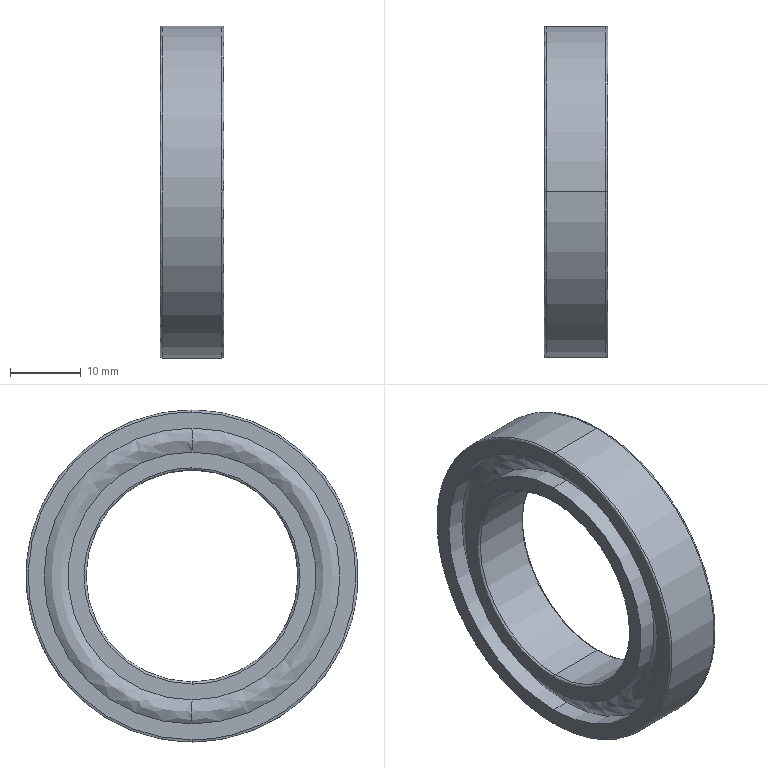Part | STEP file | radial ball bearing_68_skf_SKF - 61906 - 18,SI,NC,18_68 | 1 solid | 28 faces | box 9 x 47 x 47 mm | volume 7474 mm3 | spline 12 | cylinder 12 | plane 4 | commonest cylinder face diameters 35.1 x4 41.9 x4 30 x2 47 x2